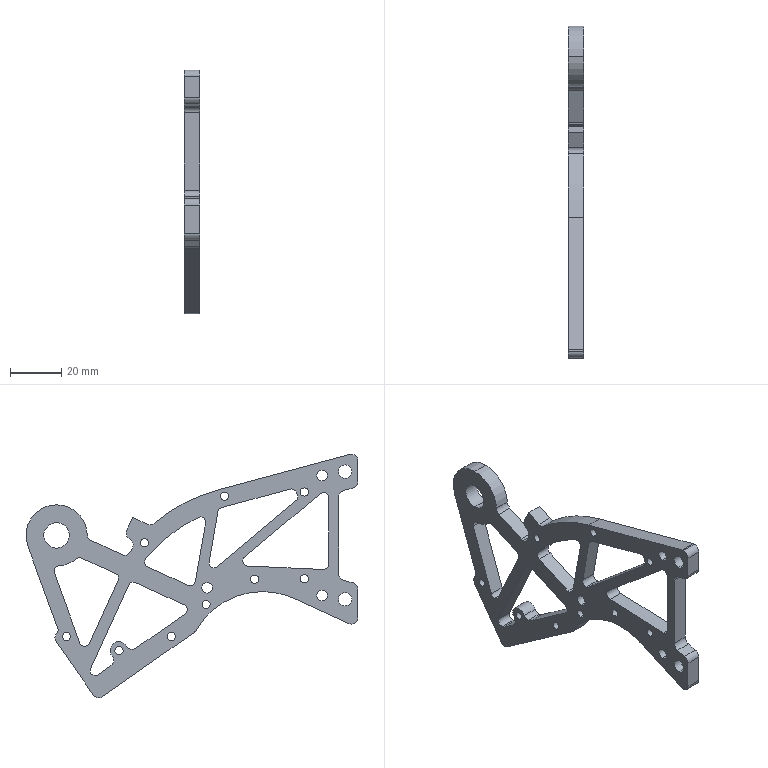Part | SolidWorks | features ICE 2, Extrusion 1, Fillet 1 | 1 solid | 112 faces | box 6 x 130 x 95.37 mm | volume 22156 mm3 | cylinder 81 | plane 31 | commonest cylinder face diameters 4 x23 3.2 x18 5 x18 4.2 x6 5.2 x4 24 x3